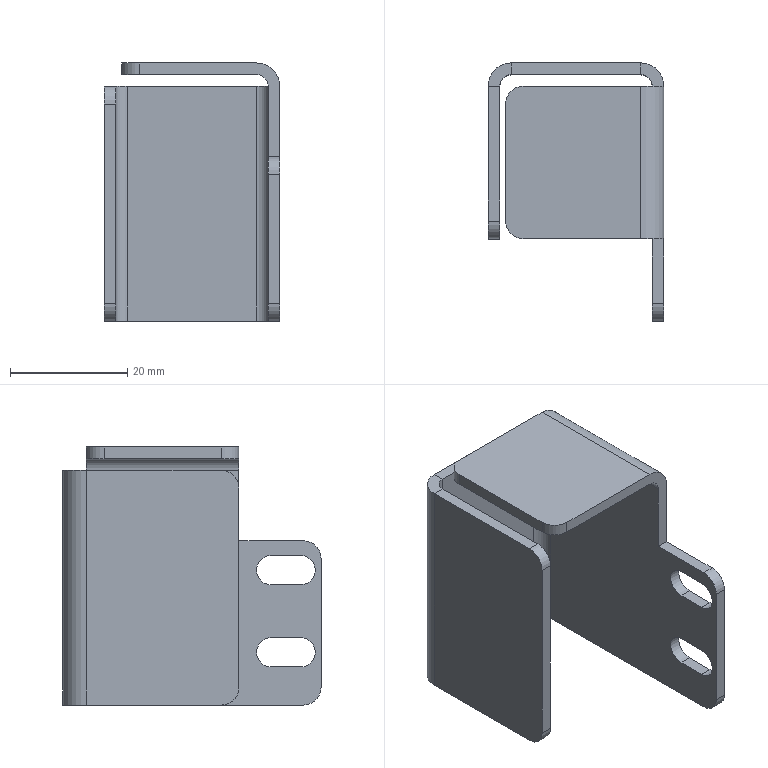Part | NX | features BREP 1 | 1 solid | 44 faces | box 30 x 44 x 44 mm | volume 8697 mm3 | plane 28 | cylinder 16 | commonest cylinder face diameters 6 x6 5 x4 4 x3 8 x3
STEP:
#1=CARTESIAN_POINT('',(-2.,42.,40.));
#2=VERTEX_POINT('',#1);
#3=CARTESIAN_POINT('',(-2.,44.,40.));
#4=VERTEX_POINT('',#3);
#5=CARTESIAN_POINT('',(-2.,42.,40.));
#6=DIRECTION('',(0.,1.,0.));
#7=VECTOR('',#6,1000.);
#8=LINE('',#5,#7);
#9=EDGE_CURVE('',#2,#4,#8,.T.);
#10=ORIENTED_EDGE('',*,*,#9,.F.);
#11=CARTESIAN_POINT('',(0.,40.,40.));
#12=VERTEX_POINT('',#11);
#13=CARTESIAN_POINT('',(-2.,40.,40.));
#14=DIRECTION('',(0.,0.,1.));
#15=DIRECTION('',(-1.,0.,0.));
#16=AXIS2_PLACEMENT_3D('',#13,#14,#15);
#17=CIRCLE('',#16,2.);
#18=EDGE_CURVE('',#12,#2,#17,.T.);
#19=ORIENTED_EDGE('',*,*,#18,.F.);
#20=CARTESIAN_POINT('',(2.,40.,40.));
#21=VERTEX_POINT('',#20);
#22=CARTESIAN_POINT('',(2.,40.,40.));
#23=DIRECTION('',(-1.,0.,0.));
#24=VECTOR('',#23,1000.);
#25=LINE('',#22,#24);
#26=EDGE_CURVE('',#21,#12,#25,.T.);
#27=ORIENTED_EDGE('',*,*,#26,.F.);
#28=CARTESIAN_POINT('',(-2.,40.,40.));
#29=DIRECTION('',(0.,0.,1.));
#30=DIRECTION('',(1.,0.,0.));
#31=AXIS2_PLACEMENT_3D('',#28,#29,#30);
#32=CIRCLE('',#31,4.);
#33=EDGE_CURVE('',#21,#4,#32,.T.);
#34=ORIENTED_EDGE('',*,*,#33,.T.);
#35=EDGE_LOOP('',(#10,#19,#27,#34));
#36=FACE_BOUND('',#35,.T.);
#37=CARTESIAN_POINT('',(-2.,42.,40.));
#38=DIRECTION('',(0.,0.,1.));
#39=DIRECTION('',(-1.,0.,0.));
#40=AXIS2_PLACEMENT_3D('',#37,#38,#39);
#41=PLANE('',#40);
#42=ADVANCED_FACE('',(#36),#41,.T.);
#43=CARTESIAN_POINT('',(-24.,42.,40.));
#44=VERTEX_POINT('',#43);
#45=CARTESIAN_POINT('',(0.,42.,40.));
#46=DIRECTION('',(-1.,0.,0.));
#47=VECTOR('',#46,1000.);
#48=LINE('',#45,#47);
#49=EDGE_CURVE('',#2,#44,#48,.T.);
#50=ORIENTED_EDGE('',*,*,#49,.F.);
#51=ORIENTED_EDGE('',*,*,#9,.T.);
#52=CARTESIAN_POINT('',(-24.,44.,40.));
#53=VERTEX_POINT('',#52);
#54=CARTESIAN_POINT('',(0.,44.,40.));
#55=DIRECTION('',(-1.,0.,0.));
#56=VECTOR('',#55,1000.);
#57=LINE('',#54,#56);
#58=EDGE_CURVE('',#4,#53,#57,.T.);
#59=ORIENTED_EDGE('',*,*,#58,.T.);
#60=CARTESIAN_POINT('',(-24.,44.,40.));
#61=DIRECTION('',(0.,-1.,0.));
#62=VECTOR('',#61,1000.);
#63=LINE('',#60,#62);
#64=EDGE_CURVE('',#53,#44,#63,.T.);
#65=ORIENTED_EDGE('',*,*,#64,.T.);
#66=EDGE_LOOP('',(#50,#51,#59,#65));
#67=FACE_BOUND('',#66,.T.);
#68=CARTESIAN_POINT('',(2.,40.,40.));
#69=DIRECTION('',(0.,0.,1.));
#70=DIRECTION('',(-1.,0.,0.));
#71=AXIS2_PLACEMENT_3D('',#68,#69,#70);
#72=PLANE('',#71);
#73=ADVANCED_FACE('',(#67),#72,.T.);
#74=CARTESIAN_POINT('',(0.,40.,0.));
#75=VERTEX_POINT('',#74);
#76=CARTESIAN_POINT('',(2.,40.,0.));
#77=VERTEX_POINT('',#76);
#78=CARTESIAN_POINT('',(0.,40.,0.));
#79=DIRECTION('',(1.,0.,0.));
#80=VECTOR('',#79,1000.);
#81=LINE('',#78,#80);
#82=EDGE_CURVE('',#75,#77,#81,.T.);
#83=ORIENTED_EDGE('',*,*,#82,.F.);
#84=CARTESIAN_POINT('',(-2.,42.,0.));
#85=VERTEX_POINT('',#84);
#86=CARTESIAN_POINT('',(-2.,40.,0.));
#87=DIRECTION('',(0.,0.,1.));
#88=DIRECTION('',(-1.,0.,0.));
#89=AXIS2_PLACEMENT_3D('',#86,#87,#88);
#90=CIRCLE('',#89,2.);
#91=EDGE_CURVE('',#75,#85,#90,.T.);
#92=ORIENTED_EDGE('',*,*,#91,.T.);
#93=CARTESIAN_POINT('',(-2.,44.,0.));
#94=VERTEX_POINT('',#93);
#95=CARTESIAN_POINT('',(-2.,44.,0.));
#96=DIRECTION('',(0.,-1.,0.));
#97=VECTOR('',#96,1000.);
#98=LINE('',#95,#97);
#99=EDGE_CURVE('',#94,#85,#98,.T.);
#100=ORIENTED_EDGE('',*,*,#99,.F.);
#101=CARTESIAN_POINT('',(-2.,40.,0.));
#102=DIRECTION('',(0.,0.,1.));
#103=DIRECTION('',(1.,0.,0.));
#104=AXIS2_PLACEMENT_3D('',#101,#102,#103);
#105=CIRCLE('',#104,4.);
#106=EDGE_CURVE('',#77,#94,#105,.T.);
#107=ORIENTED_EDGE('',*,*,#106,.F.);
#108=EDGE_LOOP('',(#83,#92,#100,#107));
#109=FACE_BOUND('',#108,.T.);
#110=CARTESIAN_POINT('',(0.,40.,0.));
#111=DIRECTION('',(0.,0.,-1.));
#112=DIRECTION('',(1.,0.,0.));
#113=AXIS2_PLACEMENT_3D('',#110,#111,#112);
#114=PLANE('',#113);
#115=ADVANCED_FACE('',(#109),#114,.T.);
#116=CARTESIAN_POINT('',(2.,3.,0.));
#117=VERTEX_POINT('',#116);
#118=CARTESIAN_POINT('',(2.,0.,0.));
#119=DIRECTION('',(0.,1.,0.));
#120=VECTOR('',#119,1000.);
#121=LINE('',#118,#120);
#122=EDGE_CURVE('',#117,#77,#121,.T.);
#123=ORIENTED_EDGE('',*,*,#122,.F.);
#124=CARTESIAN_POINT('',(0.,3.,0.));
#125=VERTEX_POINT('',#124);
#126=CARTESIAN_POINT('',(-2.,3.,0.));
#127=DIRECTION('',(-1.,0.,0.));
#128=VECTOR('',#127,1000.);
#129=LINE('',#126,#128);
#130=EDGE_CURVE('',#117,#125,#129,.T.);
#131=ORIENTED_EDGE('',*,*,#130,.T.);
#132=CARTESIAN_POINT('',(0.,0.,0.));
#133=DIRECTION('',(0.,1.,0.));
#134=VECTOR('',#133,1000.);
#135=LINE('',#132,#134);
#136=EDGE_CURVE('',#125,#75,#135,.T.);
#137=ORIENTED_EDGE('',*,*,#136,.T.);
#138=ORIENTED_EDGE('',*,*,#82,.T.);
#139=EDGE_LOOP('',(#123,#131,#137,#138));
#140=FACE_BOUND('',#139,.T.);
#141=CARTESIAN_POINT('',(-2.,44.,0.));
#142=DIRECTION('',(0.,0.,-1.));
#143=DIRECTION('',(1.,0.,0.));
#144=AXIS2_PLACEMENT_3D('',#141,#142,#143);
#145=PLANE('',#144);
#146=ADVANCED_FACE('',(#140),#145,.T.);
#147=CARTESIAN_POINT('',(-26.,40.,40.));
#148=VERTEX_POINT('',#147);
#149=CARTESIAN_POINT('',(-28.,40.,40.));
#150=VERTEX_POINT('',#149);
#151=CARTESIAN_POINT('',(-26.,40.,40.));
#152=DIRECTION('',(-1.,0.,0.));
#153=VECTOR('',#152,1000.);
#154=LINE('',#151,#153);
#155=EDGE_CURVE('',#148,#150,#154,.T.);
#156=ORIENTED_EDGE('',*,*,#155,.F.);
#157=CARTESIAN_POINT('',(-24.,40.,40.));
#158=DIRECTION('',(0.,0.,1.));
#159=DIRECTION('',(-1.,0.,0.));
#160=AXIS2_PLACEMENT_3D('',#157,#158,#159);
#161=CIRCLE('',#160,2.);
#162=EDGE_CURVE('',#44,#148,#161,.T.);
#163=ORIENTED_EDGE('',*,*,#162,.F.);
#164=ORIENTED_EDGE('',*,*,#64,.F.);
#165=CARTESIAN_POINT('',(-24.,40.,40.));
#166=DIRECTION('',(0.,0.,1.));
#167=DIRECTION('',(1.,0.,0.));
#168=AXIS2_PLACEMENT_3D('',#165,#166,#167);
#169=CIRCLE('',#168,4.);
#170=EDGE_CURVE('',#53,#150,#169,.T.);
#171=ORIENTED_EDGE('',*,*,#170,.T.);
#172=EDGE_LOOP('',(#156,#163,#164,#171));
#173=FACE_BOUND('',#172,.T.);
#174=CARTESIAN_POINT('',(-26.,40.,40.));
#175=DIRECTION('',(0.,0.,1.));
#176=DIRECTION('',(-1.,0.,0.));
#177=AXIS2_PLACEMENT_3D('',#174,#175,#176);
#178=PLANE('',#177);
#179=ADVANCED_FACE('',(#173),#178,.T.);
#180=CARTESIAN_POINT('',(-28.,17.,40.));
#181=VERTEX_POINT('',#180);
#182=CARTESIAN_POINT('',(-28.,42.,40.));
#183=DIRECTION('',(0.,-1.,0.));
#184=VECTOR('',#183,1000.);
#185=LINE('',#182,#184);
#186=EDGE_CURVE('',#150,#181,#185,.T.);
#187=ORIENTED_EDGE('',*,*,#186,.T.);
#188=CARTESIAN_POINT('',(-26.,17.,40.));
#189=VERTEX_POINT('',#188);
#190=CARTESIAN_POINT('',(-24.,17.,40.));
#191=DIRECTION('',(1.,0.,0.));
#192=VECTOR('',#191,1000.);
#193=LINE('',#190,#192);
#194=EDGE_CURVE('',#181,#189,#193,.T.);
#195=ORIENTED_EDGE('',*,*,#194,.T.);
#196=CARTESIAN_POINT('',(-26.,42.,40.));
#197=DIRECTION('',(0.,-1.,0.));
#198=VECTOR('',#197,1000.);
#199=LINE('',#196,#198);
#200=EDGE_CURVE('',#148,#189,#199,.T.);
#201=ORIENTED_EDGE('',*,*,#200,.F.);
#202=ORIENTED_EDGE('',*,*,#155,.T.);
#203=EDGE_LOOP('',(#187,#195,#201,#202));
#204=FACE_BOUND('',#203,.T.);
#205=CARTESIAN_POINT('',(-24.,44.,40.));
#206=DIRECTION('',(0.,0.,1.));
#207=DIRECTION('',(-1.,0.,0.));
#208=AXIS2_PLACEMENT_3D('',#205,#206,#207);
#209=PLANE('',#208);
#210=ADVANCED_FACE('',(#204),#209,.T.);
#211=CARTESIAN_POINT('',(-24.,42.,0.));
#212=VERTEX_POINT('',#211);
#213=CARTESIAN_POINT('',(-24.,44.,0.));
#214=VERTEX_POINT('',#213);
#215=CARTESIAN_POINT('',(-24.,42.,0.));
#216=DIRECTION('',(0.,1.,0.));
#217=VECTOR('',#216,1000.);
#218=LINE('',#215,#217);
#219=EDGE_CURVE('',#212,#214,#218,.T.);
#220=ORIENTED_EDGE('',*,*,#219,.F.);
#221=CARTESIAN_POINT('',(-26.,40.,0.));
#222=VERTEX_POINT('',#221);
#223=CARTESIAN_POINT('',(-24.,40.,0.));
#224=DIRECTION('',(0.,0.,1.));
#225=DIRECTION('',(-1.,0.,0.));
#226=AXIS2_PLACEMENT_3D('',#223,#224,#225);
#227=CIRCLE('',#226,2.);
#228=EDGE_CURVE('',#212,#222,#227,.T.);
#229=ORIENTED_EDGE('',*,*,#228,.T.);
#230=CARTESIAN_POINT('',(-28.,40.,0.));
#231=VERTEX_POINT('',#230);
#232=CARTESIAN_POINT('',(-28.,40.,0.));
#233=DIRECTION('',(1.,0.,0.));
#234=VECTOR('',#233,1000.);
#235=LINE('',#232,#234);
#236=EDGE_CURVE('',#231,#222,#235,.T.);
#237=ORIENTED_EDGE('',*,*,#236,.F.);
#238=CARTESIAN_POINT('',(-24.,40.,0.));
#239=DIRECTION('',(0.,0.,1.));
#240=DIRECTION('',(1.,0.,0.));
#241=AXIS2_PLACEMENT_3D('',#238,#239,#240);
#242=CIRCLE('',#241,4.);
#243=EDGE_CURVE('',#214,#231,#242,.T.);
#244=ORIENTED_EDGE('',*,*,#243,.F.);
#245=EDGE_LOOP('',(#220,#229,#237,#244));
#246=FACE_BOUND('',#245,.T.);
#247=CARTESIAN_POINT('',(-24.,42.,0.));
#248=DIRECTION('',(0.,0.,-1.));
#249=DIRECTION('',(1.,0.,0.));
#250=AXIS2_PLACEMENT_3D('',#247,#248,#249);
#251=PLANE('',#250);
#252=ADVANCED_FACE('',(#246),#251,.T.);
#253=CARTESIAN_POINT('',(0.,42.,0.));
#254=DIRECTION('',(-1.,0.,0.));
#255=VECTOR('',#254,1000.);
#256=LINE('',#253,#255);
#257=EDGE_CURVE('',#85,#212,#256,.T.);
#258=ORIENTED_EDGE('',*,*,#257,.T.);
#259=ORIENTED_EDGE('',*,*,#219,.T.);
#260=CARTESIAN_POINT('',(0.,44.,0.));
#261=DIRECTION('',(-1.,0.,0.));
#262=VECTOR('',#261,1000.);
#263=LINE('',#260,#262);
#264=EDGE_CURVE('',#94,#214,#263,.T.);
#265=ORIENTED_EDGE('',*,*,#264,.F.);
#266=ORIENTED_EDGE('',*,*,#99,.T.);
#267=EDGE_LOOP('',(#258,#259,#265,#266));
#268=FACE_BOUND('',#267,.T.);
#269=CARTESIAN_POINT('',(-28.,40.,0.));
#270=DIRECTION('',(0.,0.,-1.));
#271=DIRECTION('',(1.,0.,0.));
#272=AXIS2_PLACEMENT_3D('',#269,#270,#271);
#273=PLANE('',#272);
#274=ADVANCED_FACE('',(#268),#273,.T.);
#275=CARTESIAN_POINT('',(-28.,14.,37.));
#276=VERTEX_POINT('',#275);
#277=CARTESIAN_POINT('',(-28.,14.,3.));
#278=VERTEX_POINT('',#277);
#279=CARTESIAN_POINT('',(-28.,14.,40.));
#280=DIRECTION('',(0.,0.,-1.));
#281=VECTOR('',#280,1000.);
#282=LINE('',#279,#281);
#283=EDGE_CURVE('',#276,#278,#282,.T.);
#284=ORIENTED_EDGE('',*,*,#283,.F.);
#285=CARTESIAN_POINT('',(-28.,17.,37.));
#286=DIRECTION('',(-1.,0.,0.));
#287=DIRECTION('',(0.,0.,-1.));
#288=AXIS2_PLACEMENT_3D('',#285,#286,#287);
#289=CIRCLE('',#288,3.);
#290=EDGE_CURVE('',#276,#181,#289,.T.);
#291=ORIENTED_EDGE('',*,*,#290,.T.);
#292=ORIENTED_EDGE('',*,*,#186,.F.);
#293=CARTESIAN_POINT('',(-28.,40.,40.));
#294=DIRECTION('',(0.,0.,-1.));
#295=VECTOR('',#294,1000.);
#296=LINE('',#293,#295);
#297=EDGE_CURVE('',#150,#231,#296,.T.);
#298=ORIENTED_EDGE('',*,*,#297,.T.);
#299=CARTESIAN_POINT('',(-28.,17.,0.));
#300=VERTEX_POINT('',#299);
#301=CARTESIAN_POINT('',(-28.,42.,0.));
#302=DIRECTION('',(0.,-1.,0.));
#303=VECTOR('',#302,1000.);
#304=LINE('',#301,#303);
#305=EDGE_CURVE('',#231,#300,#304,.T.);
#306=ORIENTED_EDGE('',*,*,#305,.T.);
#307=CARTESIAN_POINT('',(-28.,17.,3.));
#308=DIRECTION('',(-1.,0.,0.));
#309=DIRECTION('',(0.,0.,-1.));
#310=AXIS2_PLACEMENT_3D('',#307,#308,#309);
#311=CIRCLE('',#310,3.);
#312=EDGE_CURVE('',#300,#278,#311,.T.);
#313=ORIENTED_EDGE('',*,*,#312,.T.);
#314=EDGE_LOOP('',(#284,#291,#292,#298,#306,#313));
#315=FACE_BOUND('',#314,.T.);
#316=CARTESIAN_POINT('',(-28.,42.,40.));
#317=DIRECTION('',(1.,0.,0.));
#318=DIRECTION('',(0.,0.,1.));
#319=AXIS2_PLACEMENT_3D('',#316,#317,#318);
#320=PLANE('',#319);
#321=ADVANCED_FACE('',(#315),#320,.F.);
#322=CARTESIAN_POINT('',(-26.,14.,37.));
#323=VERTEX_POINT('',#322);
#324=CARTESIAN_POINT('',(-26.,14.,3.));
#325=VERTEX_POINT('',#324);
#326=CARTESIAN_POINT('',(-26.,14.,40.));
#327=DIRECTION('',(0.,0.,-1.));
#328=VECTOR('',#327,1000.);
#329=LINE('',#326,#328);
#330=EDGE_CURVE('',#323,#325,#329,.T.);
#331=ORIENTED_EDGE('',*,*,#330,.F.);
#332=CARTESIAN_POINT('',(-26.,14.,37.));
#333=DIRECTION('',(-1.,0.,0.));
#334=VECTOR('',#333,1000.);
#335=LINE('',#332,#334);
#336=EDGE_CURVE('',#323,#276,#335,.T.);
#337=ORIENTED_EDGE('',*,*,#336,.T.);
#338=ORIENTED_EDGE('',*,*,#283,.T.);
#339=CARTESIAN_POINT('',(-26.,14.,3.));
#340=DIRECTION('',(1.,0.,0.));
#341=VECTOR('',#340,1000.);
#342=LINE('',#339,#341);
#343=EDGE_CURVE('',#278,#325,#342,.T.);
#344=ORIENTED_EDGE('',*,*,#343,.T.);
#345=EDGE_LOOP('',(#331,#337,#338,#344));
#346=FACE_BOUND('',#345,.T.);
#347=CARTESIAN_POINT('',(-26.,14.,40.));
#348=DIRECTION('',(0.,-1.,0.));
#349=DIRECTION('',(0.,0.,1.));
#350=AXIS2_PLACEMENT_3D('',#347,#348,#349);
#351=PLANE('',#350);
#352=ADVANCED_FACE('',(#346),#351,.T.);
#353=ORIENTED_EDGE('',*,*,#200,.T.);
#354=CARTESIAN_POINT('',(-26.,17.,37.));
#355=DIRECTION('',(1.,0.,0.));
#356=DIRECTION('',(0.,0.,-1.));
#357=AXIS2_PLACEMENT_3D('',#354,#355,#356);
#358=CIRCLE('',#357,3.);
#359=EDGE_CURVE('',#189,#323,#358,.T.);
#360=ORIENTED_EDGE('',*,*,#359,.T.);
#361=ORIENTED_EDGE('',*,*,#330,.T.);
#362=CARTESIAN_POINT('',(-26.,17.,0.));
#363=VERTEX_POINT('',#362);
#364=CARTESIAN_POINT('',(-26.,17.,3.));
#365=DIRECTION('',(1.,0.,0.));
#366=DIRECTION('',(0.,0.,-1.));
#367=AXIS2_PLACEMENT_3D('',#364,#365,#366);
#368=CIRCLE('',#367,3.);
#369=EDGE_CURVE('',#325,#363,#368,.T.);
#370=ORIENTED_EDGE('',*,*,#369,.T.);
#371=CARTESIAN_POINT('',(-26.,42.,0.));
#372=DIRECTION('',(0.,-1.,0.));
#373=VECTOR('',#372,1000.);
#374=LINE('',#371,#373);
#375=EDGE_CURVE('',#222,#363,#374,.T.);
#376=ORIENTED_EDGE('',*,*,#375,.F.);
#377=CARTESIAN_POINT('',(-26.,40.,40.));
#378=DIRECTION('',(0.,0.,-1.));
#379=VECTOR('',#378,1000.);
#380=LINE('',#377,#379);
#381=EDGE_CURVE('',#148,#222,#380,.T.);
#382=ORIENTED_EDGE('',*,*,#381,.F.);
#383=EDGE_LOOP('',(#353,#360,#361,#370,#376,#382));
#384=FACE_BOUND('',#383,.T.);
#385=CARTESIAN_POINT('',(-26.,42.,40.));
#386=DIRECTION('',(1.,0.,0.));
#387=DIRECTION('',(0.,0.,1.));
#388=AXIS2_PLACEMENT_3D('',#385,#386,#387);
#389=PLANE('',#388);
#390=ADVANCED_FACE('',(#384),#389,.T.);
#391=ORIENTED_EDGE('',*,*,#228,.F.);
#392=CARTESIAN_POINT('',(-24.,42.,40.));
#393=DIRECTION('',(0.,0.,-1.));
#394=VECTOR('',#393,1000.);
#395=LINE('',#392,#394);
#396=EDGE_CURVE('',#44,#212,#395,.T.);
#397=ORIENTED_EDGE('',*,*,#396,.F.);
#398=ORIENTED_EDGE('',*,*,#162,.T.);
#399=ORIENTED_EDGE('',*,*,#381,.T.);
#400=EDGE_LOOP('',(#391,#397,#398,#399));
#401=FACE_BOUND('',#400,.T.);
#402=CARTESIAN_POINT('',(-24.,40.,40.));
#403=DIRECTION('',(0.,0.,-1.));
#404=DIRECTION('',(1.,0.,0.));
#405=AXIS2_PLACEMENT_3D('',#402,#403,#404);
#406=CYLINDRICAL_SURFACE('',#405,2.);
#407=ADVANCED_FACE('',(#401),#406,.F.);
#408=ORIENTED_EDGE('',*,*,#257,.F.);
#409=CARTESIAN_POINT('',(-2.,42.,40.));
#410=DIRECTION('',(0.,0.,-1.));
#411=VECTOR('',#410,1000.);
#412=LINE('',#409,#411);
#413=EDGE_CURVE('',#2,#85,#412,.T.);
#414=ORIENTED_EDGE('',*,*,#413,.F.);
#415=ORIENTED_EDGE('',*,*,#49,.T.);
#416=ORIENTED_EDGE('',*,*,#396,.T.);
#417=EDGE_LOOP('',(#408,#414,#415,#416));
#418=FACE_BOUND('',#417,.T.);
#419=CARTESIAN_POINT('',(0.,42.,40.));
#420=DIRECTION('',(0.,-1.,0.));
#421=DIRECTION('',(-1.,0.,0.));
#422=AXIS2_PLACEMENT_3D('',#419,#420,#421);
#423=PLANE('',#422);
#424=ADVANCED_FACE('',(#418),#423,.T.);
#425=ORIENTED_EDGE('',*,*,#91,.F.);
#426=CARTESIAN_POINT('',(0.,40.,40.));
#427=DIRECTION('',(0.,0.,-1.));
#428=VECTOR('',#427,1000.);
#429=LINE('',#426,#428);
#430=EDGE_CURVE('',#12,#75,#429,.T.);
#431=ORIENTED_EDGE('',*,*,#430,.F.);
#432=ORIENTED_EDGE('',*,*,#18,.T.);
#433=ORIENTED_EDGE('',*,*,#413,.T.);
#434=EDGE_LOOP('',(#425,#431,#432,#433));
#435=FACE_BOUND('',#434,.T.);
#436=CARTESIAN_POINT('',(-2.,40.,40.));
#437=DIRECTION('',(0.,0.,-1.));
#438=DIRECTION('',(1.,0.,0.));
#439=AXIS2_PLACEMENT_3D('',#436,#437,#438);
#440=CYLINDRICAL_SURFACE('',#439,2.);
#441=ADVANCED_FACE('',(#435),#440,.F.);
#442=CARTESIAN_POINT('',(0.,8.5,25.5));
#443=VERTEX_POINT('',#442);
#444=CARTESIAN_POINT('',(0.,8.5,20.5));
#445=VERTEX_POINT('',#444);
#446=CARTESIAN_POINT('',(0.,8.5,23.));
#447=DIRECTION('',(-1.,0.,0.));
#448=DIRECTION('',(0.,0.,1.));
#449=AXIS2_PLACEMENT_3D('',#446,#447,#448);
#450=CIRCLE('',#449,2.5);
#451=EDGE_CURVE('',#443,#445,#450,.T.);
#452=ORIENTED_EDGE('',*,*,#451,.F.);
#453=CARTESIAN_POINT('',(0.,3.5,25.5));
#454=VERTEX_POINT('',#453);
#455=CARTESIAN_POINT('',(0.,0.,25.5));
#456=DIRECTION('',(0.,1.,0.));
#457=VECTOR('',#456,1000.);
#458=LINE('',#455,#457);
#459=EDGE_CURVE('',#454,#443,#458,.T.);
#460=ORIENTED_EDGE('',*,*,#459,.F.);
#461=CARTESIAN_POINT('',(0.,3.5,20.5));
#462=VERTEX_POINT('',#461);
#463=CARTESIAN_POINT('',(0.,3.5,23.));
#464=DIRECTION('',(-1.,0.,0.));
#465=DIRECTION('',(0.,0.,1.));
#466=AXIS2_PLACEMENT_3D('',#463,#464,#465);
#467=CIRCLE('',#466,2.5);
#468=EDGE_CURVE('',#462,#454,#467,.T.);
#469=ORIENTED_EDGE('',*,*,#468,.F.);
#470=CARTESIAN_POINT('',(0.,0.,20.5));
#471=DIRECTION('',(0.,-1.,0.));
#472=VECTOR('',#471,1000.);
#473=LINE('',#470,#472);
#474=EDGE_CURVE('',#445,#462,#473,.T.);
#475=ORIENTED_EDGE('',*,*,#474,.F.);
#476=EDGE_LOOP('',(#452,#460,#469,#475));
#477=FACE_BOUND('',#476,.T.);
#478=CARTESIAN_POINT('',(0.,8.5,11.5));
#479=VERTEX_POINT('',#478);
#480=CARTESIAN_POINT('',(0.,8.5,6.5));
#481=VERTEX_POINT('',#480);
#482=CARTESIAN_POINT('',(0.,8.5,9.));
#483=DIRECTION('',(-1.,0.,0.));
#484=DIRECTION('',(0.,0.,1.));
#485=AXIS2_PLACEMENT_3D('',#482,#483,#484);
#486=CIRCLE('',#485,2.5);
#487=EDGE_CURVE('',#479,#481,#486,.T.);
#488=ORIENTED_EDGE('',*,*,#487,.F.);
#489=CARTESIAN_POINT('',(0.,3.5,11.5));
#490=VERTEX_POINT('',#489);
#491=CARTESIAN_POINT('',(0.,0.,11.5));
#492=DIRECTION('',(0.,1.,0.));
#493=VECTOR('',#492,1000.);
#494=LINE('',#491,#493);
#495=EDGE_CURVE('',#490,#479,#494,.T.);
#496=ORIENTED_EDGE('',*,*,#495,.F.);
#497=CARTESIAN_POINT('',(0.,3.5,6.5));
#498=VERTEX_POINT('',#497);
#499=CARTESIAN_POINT('',(0.,3.5,9.));
#500=DIRECTION('',(-1.,0.,0.));
#501=DIRECTION('',(0.,0.,1.));
#502=AXIS2_PLACEMENT_3D('',#499,#500,#501);
#503=CIRCLE('',#502,2.5);
#504=EDGE_CURVE('',#498,#490,#503,.T.);
#505=ORIENTED_EDGE('',*,*,#504,.F.);
#506=CARTESIAN_POINT('',(0.,0.,6.5));
#507=DIRECTION('',(0.,-1.,0.));
#508=VECTOR('',#507,1000.);
#509=LINE('',#506,#508);
#510=EDGE_CURVE('',#481,#498,#509,.T.);
#511=ORIENTED_EDGE('',*,*,#510,.F.);
#512=EDGE_LOOP('',(#488,#496,#505,#511));
#513=FACE_BOUND('',#512,.T.);
#514=ORIENTED_EDGE('',*,*,#136,.F.);
#515=CARTESIAN_POINT('',(0.,0.,3.));
#516=VERTEX_POINT('',#515);
#517=CARTESIAN_POINT('',(0.,3.,3.));
#518=DIRECTION('',(-1.,0.,0.));
#519=DIRECTION('',(0.,0.,1.));
#520=AXIS2_PLACEMENT_3D('',#517,#518,#519);
#521=CIRCLE('',#520,3.);
#522=EDGE_CURVE('',#125,#516,#521,.T.);
#523=ORIENTED_EDGE('',*,*,#522,.T.);
#524=CARTESIAN_POINT('',(0.,0.,25.));
#525=VERTEX_POINT('',#524);
#526=CARTESIAN_POINT('',(0.,0.,40.));
#527=DIRECTION('',(0.,0.,-1.));
#528=VECTOR('',#527,1000.);
#529=LINE('',#526,#528);
#530=EDGE_CURVE('',#525,#516,#529,.T.);
#531=ORIENTED_EDGE('',*,*,#530,.F.);
#532=CARTESIAN_POINT('',(0.,3.,28.));
#533=VERTEX_POINT('',#532);
#534=CARTESIAN_POINT('',(0.,3.,25.));
#535=DIRECTION('',(-1.,0.,0.));
#536=DIRECTION('',(0.,0.,1.));
#537=AXIS2_PLACEMENT_3D('',#534,#535,#536);
#538=CIRCLE('',#537,3.);
#539=EDGE_CURVE('',#525,#533,#538,.T.);
#540=ORIENTED_EDGE('',*,*,#539,.T.);
#541=CARTESIAN_POINT('',(0.,14.,28.));
#542=VERTEX_POINT('',#541);
#543=CARTESIAN_POINT('',(0.,0.,28.));
#544=DIRECTION('',(0.,-1.,0.));
#545=VECTOR('',#544,1000.);
#546=LINE('',#543,#545);
#547=EDGE_CURVE('',#542,#533,#546,.T.);
#548=ORIENTED_EDGE('',*,*,#547,.F.);
#549=CARTESIAN_POINT('',(0.,14.,40.));
#550=VERTEX_POINT('',#549);
#551=CARTESIAN_POINT('',(0.,14.,40.));
#552=DIRECTION('',(0.,0.,-1.));
#553=VECTOR('',#552,1000.);
#554=LINE('',#551,#553);
#555=EDGE_CURVE('',#550,#542,#554,.T.);
#556=ORIENTED_EDGE('',*,*,#555,.F.);
#557=CARTESIAN_POINT('',(0.,0.,40.));
#558=DIRECTION('',(0.,1.,0.));
#559=VECTOR('',#558,1000.);
#560=LINE('',#557,#559);
#561=EDGE_CURVE('',#550,#12,#560,.T.);
#562=ORIENTED_EDGE('',*,*,#561,.T.);
#563=ORIENTED_EDGE('',*,*,#430,.T.);
#564=EDGE_LOOP('',(#514,#523,#531,#540,#548,#556,#562,#563));
#565=FACE_BOUND('',#564,.T.);
#566=CARTESIAN_POINT('',(0.,0.,40.));
#567=DIRECTION('',(-1.,0.,0.));
#568=DIRECTION('',(0.,0.,-1.));
#569=AXIS2_PLACEMENT_3D('',#566,#567,#568);
#570=PLANE('',#569);
#571=ADVANCED_FACE('',(#477,#513,#565),#570,.T.);
#572=ORIENTED_EDGE('',*,*,#530,.T.);
#573=CARTESIAN_POINT('',(2.,0.,3.));
#574=VERTEX_POINT('',#573);
#575=CARTESIAN_POINT('',(2.,0.,3.));
#576=DIRECTION('',(1.,0.,0.));
#577=VECTOR('',#576,1000.);
#578=LINE('',#575,#577);
#579=EDGE_CURVE('',#516,#574,#578,.T.);
#580=ORIENTED_EDGE('',*,*,#579,.T.);
#581=CARTESIAN_POINT('',(2.,0.,25.));
#582=VERTEX_POINT('',#581);
#583=CARTESIAN_POINT('',(2.,0.,40.));
#584=DIRECTION('',(0.,0.,-1.));
#585=VECTOR('',#584,1000.);
#586=LINE('',#583,#585);
#587=EDGE_CURVE('',#582,#574,#586,.T.);
#588=ORIENTED_EDGE('',*,*,#587,.F.);
#589=CARTESIAN_POINT('',(0.,0.,25.));
#590=DIRECTION('',(-1.,0.,0.));
#591=VECTOR('',#590,1000.);
#592=LINE('',#589,#591);
#593=EDGE_CURVE('',#582,#525,#592,.T.);
#594=ORIENTED_EDGE('',*,*,#593,.T.);
#595=EDGE_LOOP('',(#572,#580,#588,#594));
#596=FACE_BOUND('',#595,.T.);
#597=CARTESIAN_POINT('',(2.,0.,40.));
#598=DIRECTION('',(0.,-1.,0.));
#599=DIRECTION('',(0.,0.,1.));
#600=AXIS2_PLACEMENT_3D('',#597,#598,#599);
#601=PLANE('',#600);
#602=ADVANCED_FACE('',(#596),#601,.T.);
#603=CARTESIAN_POINT('',(2.,8.5,25.5));
#604=VERTEX_POINT('',#603);
#605=CARTESIAN_POINT('',(2.,3.5,25.5));
#606=VERTEX_POINT('',#605);
#607=CARTESIAN_POINT('',(2.,8.5,25.5));
#608=DIRECTION('',(0.,-1.,0.));
#609=VECTOR('',#608,1000.);
#610=LINE('',#607,#609);
#611=EDGE_CURVE('',#604,#606,#610,.T.);
#612=ORIENTED_EDGE('',*,*,#611,.F.);
#613=CARTESIAN_POINT('',(2.,8.5,20.5));
#614=VERTEX_POINT('',#613);
#615=CARTESIAN_POINT('',(2.,8.5,23.));
#616=DIRECTION('',(1.,0.,0.));
#617=DIRECTION('',(0.,0.,-1.));
#618=AXIS2_PLACEMENT_3D('',#615,#616,#617);
#619=CIRCLE('',#618,2.5);
#620=EDGE_CURVE('',#614,#604,#619,.T.);
#621=ORIENTED_EDGE('',*,*,#620,.F.);
#622=CARTESIAN_POINT('',(2.,3.5,20.5));
#623=VERTEX_POINT('',#622);
#624=CARTESIAN_POINT('',(2.,8.5,20.5));
#625=DIRECTION('',(0.,1.,0.));
#626=VECTOR('',#625,1000.);
#627=LINE('',#624,#626);
#628=EDGE_CURVE('',#623,#614,#627,.T.);
#629=ORIENTED_EDGE('',*,*,#628,.F.);
#630=CARTESIAN_POINT('',(2.,3.5,23.));
#631=DIRECTION('',(1.,0.,0.));
#632=DIRECTION('',(0.,0.,-1.));
#633=AXIS2_PLACEMENT_3D('',#630,#631,#632);
#634=CIRCLE('',#633,2.5);
#635=EDGE_CURVE('',#606,#623,#634,.T.);
#636=ORIENTED_EDGE('',*,*,#635,.F.);
#637=EDGE_LOOP('',(#612,#621,#629,#636));
#638=FACE_BOUND('',#637,.T.);
#639=CARTESIAN_POINT('',(2.,8.5,11.5));
#640=VERTEX_POINT('',#639);
#641=CARTESIAN_POINT('',(2.,3.5,11.5));
#642=VERTEX_POINT('',#641);
#643=CARTESIAN_POINT('',(2.,8.5,11.5));
#644=DIRECTION('',(0.,-1.,0.));
#645=VECTOR('',#644,1000.);
#646=LINE('',#643,#645);
#647=EDGE_CURVE('',#640,#642,#646,.T.);
#648=ORIENTED_EDGE('',*,*,#647,.F.);
#649=CARTESIAN_POINT('',(2.,8.5,6.5));
#650=VERTEX_POINT('',#649);
#651=CARTESIAN_POINT('',(2.,8.5,9.));
#652=DIRECTION('',(1.,0.,0.));
#653=DIRECTION('',(0.,0.,-1.));
#654=AXIS2_PLACEMENT_3D('',#651,#652,#653);
#655=CIRCLE('',#654,2.5);
#656=EDGE_CURVE('',#650,#640,#655,.T.);
#657=ORIENTED_EDGE('',*,*,#656,.F.);
#658=CARTESIAN_POINT('',(2.,3.5,6.5));
#659=VERTEX_POINT('',#658);
#660=CARTESIAN_POINT('',(2.,8.5,6.5));
#661=DIRECTION('',(0.,1.,0.));
#662=VECTOR('',#661,1000.);
#663=LINE('',#660,#662);
#664=EDGE_CURVE('',#659,#650,#663,.T.);
#665=ORIENTED_EDGE('',*,*,#664,.F.);
#666=CARTESIAN_POINT('',(2.,3.5,9.));
#667=DIRECTION('',(1.,0.,0.));
#668=DIRECTION('',(0.,0.,-1.));
#669=AXIS2_PLACEMENT_3D('',#666,#667,#668);
#670=CIRCLE('',#669,2.5);
#671=EDGE_CURVE('',#642,#659,#670,.T.);
#672=ORIENTED_EDGE('',*,*,#671,.F.);
#673=EDGE_LOOP('',(#648,#657,#665,#672));
#674=FACE_BOUND('',#673,.T.);
#675=ORIENTED_EDGE('',*,*,#587,.T.);
#676=CARTESIAN_POINT('',(2.,3.,3.));
#677=DIRECTION('',(1.,0.,0.));
#678=DIRECTION('',(0.,0.,1.));
#679=AXIS2_PLACEMENT_3D('',#676,#677,#678);
#680=CIRCLE('',#679,3.);
#681=EDGE_CURVE('',#574,#117,#680,.T.);
#682=ORIENTED_EDGE('',*,*,#681,.T.);
#683=ORIENTED_EDGE('',*,*,#122,.T.);
#684=CARTESIAN_POINT('',(2.,40.,40.));
#685=DIRECTION('',(0.,0.,-1.));
#686=VECTOR('',#685,1000.);
#687=LINE('',#684,#686);
#688=EDGE_CURVE('',#21,#77,#687,.T.);
#689=ORIENTED_EDGE('',*,*,#688,.F.);
#690=CARTESIAN_POINT('',(2.,14.,40.));
#691=VERTEX_POINT('',#690);
#692=CARTESIAN_POINT('',(2.,0.,40.));
#693=DIRECTION('',(0.,1.,0.));
#694=VECTOR('',#693,1000.);
#695=LINE('',#692,#694);
#696=EDGE_CURVE('',#691,#21,#695,.T.);
#697=ORIENTED_EDGE('',*,*,#696,.F.);
#698=CARTESIAN_POINT('',(2.,14.,28.));
#699=VERTEX_POINT('',#698);
#700=CARTESIAN_POINT('',(2.,14.,28.));
#701=DIRECTION('',(0.,0.,1.));
#702=VECTOR('',#701,1000.);
#703=LINE('',#700,#702);
#704=EDGE_CURVE('',#699,#691,#703,.T.);
#705=ORIENTED_EDGE('',*,*,#704,.F.);
#706=CARTESIAN_POINT('',(2.,3.,28.));
#707=VERTEX_POINT('',#706);
#708=CARTESIAN_POINT('',(2.,14.,28.));
#709=DIRECTION('',(0.,1.,0.));
#710=VECTOR('',#709,1000.);
#711=LINE('',#708,#710);
#712=EDGE_CURVE('',#707,#699,#711,.T.);
#713=ORIENTED_EDGE('',*,*,#712,.F.);
#714=CARTESIAN_POINT('',(2.,3.,25.));
#715=DIRECTION('',(1.,0.,0.));
#716=DIRECTION('',(0.,0.,1.));
#717=AXIS2_PLACEMENT_3D('',#714,#715,#716);
#718=CIRCLE('',#717,3.);
#719=EDGE_CURVE('',#707,#582,#718,.T.);
#720=ORIENTED_EDGE('',*,*,#719,.T.);
#721=EDGE_LOOP('',(#675,#682,#683,#689,#697,#705,#713,#720));
#722=FACE_BOUND('',#721,.T.);
#723=CARTESIAN_POINT('',(2.,0.,40.));
#724=DIRECTION('',(-1.,0.,0.));
#725=DIRECTION('',(0.,0.,-1.));
#726=AXIS2_PLACEMENT_3D('',#723,#724,#725);
#727=PLANE('',#726);
#728=ADVANCED_FACE('',(#638,#674,#722),#727,.F.);
#729=ORIENTED_EDGE('',*,*,#106,.T.);
#730=CARTESIAN_POINT('',(-2.,44.,40.));
#731=DIRECTION('',(0.,0.,-1.));
#732=VECTOR('',#731,1000.);
#733=LINE('',#730,#732);
#734=EDGE_CURVE('',#4,#94,#733,.T.);
#735=ORIENTED_EDGE('',*,*,#734,.F.);
#736=ORIENTED_EDGE('',*,*,#33,.F.);
#737=ORIENTED_EDGE('',*,*,#688,.T.);
#738=EDGE_LOOP('',(#729,#735,#736,#737));
#739=FACE_BOUND('',#738,.T.);
#740=CARTESIAN_POINT('',(-2.,40.,40.));
#741=DIRECTION('',(0.,0.,-1.));
#742=DIRECTION('',(1.,0.,0.));
#743=AXIS2_PLACEMENT_3D('',#740,#741,#742);
#744=CYLINDRICAL_SURFACE('',#743,4.);
#745=ADVANCED_FACE('',(#739),#744,.T.);
#746=ORIENTED_EDGE('',*,*,#264,.T.);
#747=CARTESIAN_POINT('',(-24.,44.,40.));
#748=DIRECTION('',(0.,0.,-1.));
#749=VECTOR('',#748,1000.);
#750=LINE('',#747,#749);
#751=EDGE_CURVE('',#53,#214,#750,.T.);
#752=ORIENTED_EDGE('',*,*,#751,.F.);
#753=ORIENTED_EDGE('',*,*,#58,.F.);
#754=ORIENTED_EDGE('',*,*,#734,.T.);
#755=EDGE_LOOP('',(#746,#752,#753,#754));
#756=FACE_BOUND('',#755,.T.);
#757=CARTESIAN_POINT('',(0.,44.,40.));
#758=DIRECTION('',(0.,-1.,0.));
#759=DIRECTION('',(-1.,0.,0.));
#760=AXIS2_PLACEMENT_3D('',#757,#758,#759);
#761=PLANE('',#760);
#762=ADVANCED_FACE('',(#756),#761,.F.);
#763=ORIENTED_EDGE('',*,*,#243,.T.);
#764=ORIENTED_EDGE('',*,*,#297,.F.);
#765=ORIENTED_EDGE('',*,*,#170,.F.);
#766=ORIENTED_EDGE('',*,*,#751,.T.);
#767=EDGE_LOOP('',(#763,#764,#765,#766));
#768=FACE_BOUND('',#767,.T.);
#769=CARTESIAN_POINT('',(-24.,40.,40.));
#770=DIRECTION('',(0.,0.,-1.));
#771=DIRECTION('',(1.,0.,0.));
#772=AXIS2_PLACEMENT_3D('',#769,#770,#771);
#773=CYLINDRICAL_SURFACE('',#772,4.);
#774=ADVANCED_FACE('',(#768),#773,.T.);
#775=ORIENTED_EDGE('',*,*,#375,.T.);
#776=CARTESIAN_POINT('',(-24.,17.,0.));
#777=DIRECTION('',(-1.,0.,0.));
#778=VECTOR('',#777,1000.);
#779=LINE('',#776,#778);
#780=EDGE_CURVE('',#363,#300,#779,.T.);
#781=ORIENTED_EDGE('',*,*,#780,.T.);
#782=ORIENTED_EDGE('',*,*,#305,.F.);
#783=ORIENTED_EDGE('',*,*,#236,.T.);
#784=EDGE_LOOP('',(#775,#781,#782,#783));
#785=FACE_BOUND('',#784,.T.);
#786=CARTESIAN_POINT('',(-24.,40.,0.));
#787=DIRECTION('',(0.,0.,-1.));
#788=DIRECTION('',(1.,0.,0.));
#789=AXIS2_PLACEMENT_3D('',#786,#787,#788);
#790=PLANE('',#789);
#791=ADVANCED_FACE('',(#785),#790,.T.);
#792=CARTESIAN_POINT('',(-2.,40.,42.));
#793=VERTEX_POINT('',#792);
#794=CARTESIAN_POINT('',(-2.,40.,40.));
#795=DIRECTION('',(0.,1.,0.));
#796=DIRECTION('',(0.,0.,1.));
#797=AXIS2_PLACEMENT_3D('',#794,#795,#796);
#798=CIRCLE('',#797,2.);
#799=EDGE_CURVE('',#793,#12,#798,.T.);
#800=ORIENTED_EDGE('',*,*,#799,.F.);
#801=CARTESIAN_POINT('',(-2.,40.,44.));
#802=VERTEX_POINT('',#801);
#803=CARTESIAN_POINT('',(-2.,40.,42.));
#804=DIRECTION('',(0.,0.,1.));
#805=VECTOR('',#804,1000.);
#806=LINE('',#803,#805);
#807=EDGE_CURVE('',#793,#802,#806,.T.);
#808=ORIENTED_EDGE('',*,*,#807,.T.);
#809=CARTESIAN_POINT('',(-2.,40.,40.));
#810=DIRECTION('',(0.,1.,0.));
#811=DIRECTION('',(0.,0.,1.));
#812=AXIS2_PLACEMENT_3D('',#809,#810,#811);
#813=CIRCLE('',#812,4.);
#814=EDGE_CURVE('',#802,#21,#813,.T.);
#815=ORIENTED_EDGE('',*,*,#814,.T.);
#816=ORIENTED_EDGE('',*,*,#26,.T.);
#817=EDGE_LOOP('',(#800,#808,#815,#816));
#818=FACE_BOUND('',#817,.T.);
#819=CARTESIAN_POINT('',(-2.,40.,40.));
#820=DIRECTION('',(0.,-1.,0.));
#821=DIRECTION('',(0.,0.,1.));
#822=AXIS2_PLACEMENT_3D('',#819,#820,#821);
#823=PLANE('',#822);
#824=ADVANCED_FACE('',(#818),#823,.F.);
#825=CARTESIAN_POINT('',(-2.,14.,44.));
#826=VERTEX_POINT('',#825);
#827=CARTESIAN_POINT('',(-2.,14.,40.));
#828=DIRECTION('',(0.,-1.,0.));
#829=DIRECTION('',(-1.,0.,0.));
#830=AXIS2_PLACEMENT_3D('',#827,#828,#829);
#831=CIRCLE('',#830,4.);
#832=EDGE_CURVE('',#691,#826,#831,.T.);
#833=ORIENTED_EDGE('',*,*,#832,.F.);
#834=ORIENTED_EDGE('',*,*,#696,.T.);
#835=ORIENTED_EDGE('',*,*,#814,.F.);
#836=CARTESIAN_POINT('',(-2.,0.,44.));
#837=DIRECTION('',(0.,-1.,0.));
#838=VECTOR('',#837,1000.);
#839=LINE('',#836,#838);
#840=EDGE_CURVE('',#802,#826,#839,.T.);
#841=ORIENTED_EDGE('',*,*,#840,.T.);
#842=EDGE_LOOP('',(#833,#834,#835,#841));
#843=FACE_BOUND('',#842,.T.);
#844=CARTESIAN_POINT('',(-2.,40.,40.));
#845=DIRECTION('',(0.,1.,0.));
#846=DIRECTION('',(0.,0.,-1.));
#847=AXIS2_PLACEMENT_3D('',#844,#845,#846);
#848=CYLINDRICAL_SURFACE('',#847,4.);
#849=ADVANCED_FACE('',(#843),#848,.T.);
#850=ORIENTED_EDGE('',*,*,#561,.F.);
#851=CARTESIAN_POINT('',(-2.,14.,42.));
#852=VERTEX_POINT('',#851);
#853=CARTESIAN_POINT('',(-2.,14.,40.));
#854=DIRECTION('',(0.,-1.,0.));
#855=DIRECTION('',(-1.,0.,0.));
#856=AXIS2_PLACEMENT_3D('',#853,#854,#855);
#857=CIRCLE('',#856,2.);
#858=EDGE_CURVE('',#550,#852,#857,.T.);
#859=ORIENTED_EDGE('',*,*,#858,.T.);
#860=CARTESIAN_POINT('',(-2.,0.,42.));
#861=DIRECTION('',(0.,1.,0.));
#862=VECTOR('',#861,1000.);
#863=LINE('',#860,#862);
#864=EDGE_CURVE('',#852,#793,#863,.T.);
#865=ORIENTED_EDGE('',*,*,#864,.T.);
#866=ORIENTED_EDGE('',*,*,#799,.T.);
#867=EDGE_LOOP('',(#850,#859,#865,#866));
#868=FACE_BOUND('',#867,.T.);
#869=CARTESIAN_POINT('',(-2.,40.,40.));
#870=DIRECTION('',(0.,1.,0.));
#871=DIRECTION('',(0.,0.,-1.));
#872=AXIS2_PLACEMENT_3D('',#869,#870,#871);
#873=CYLINDRICAL_SURFACE('',#872,2.);
#874=ADVANCED_FACE('',(#868),#873,.F.);
#875=CARTESIAN_POINT('',(-22.,40.,42.));
#876=VERTEX_POINT('',#875);
#877=CARTESIAN_POINT('',(-25.,40.,42.));
#878=DIRECTION('',(-1.,0.,0.));
#879=VECTOR('',#878,1000.);
#880=LINE('',#877,#879);
#881=EDGE_CURVE('',#793,#876,#880,.T.);
#882=ORIENTED_EDGE('',*,*,#881,.T.);
#883=CARTESIAN_POINT('',(-22.,40.,44.));
#884=VERTEX_POINT('',#883);
#885=CARTESIAN_POINT('',(-22.,40.,44.));
#886=DIRECTION('',(0.,0.,1.));
#887=VECTOR('',#886,1000.);
#888=LINE('',#885,#887);
#889=EDGE_CURVE('',#876,#884,#888,.T.);
#890=ORIENTED_EDGE('',*,*,#889,.T.);
#891=CARTESIAN_POINT('',(0.,40.,44.));
#892=DIRECTION('',(-1.,0.,0.));
#893=VECTOR('',#892,1000.);
#894=LINE('',#891,#893);
#895=EDGE_CURVE('',#802,#884,#894,.T.);
#896=ORIENTED_EDGE('',*,*,#895,.F.);
#897=ORIENTED_EDGE('',*,*,#807,.F.);
#898=EDGE_LOOP('',(#882,#890,#896,#897));
#899=FACE_BOUND('',#898,.T.);
#900=CARTESIAN_POINT('',(-25.,40.,44.));
#901=DIRECTION('',(0.,-1.,0.));
#902=DIRECTION('',(0.,0.,1.));
#903=AXIS2_PLACEMENT_3D('',#900,#901,#902);
#904=PLANE('',#903);
#905=ADVANCED_FACE('',(#899),#904,.F.);
#906=ORIENTED_EDGE('',*,*,#895,.T.);
#907=CARTESIAN_POINT('',(-25.,37.,44.));
#908=VERTEX_POINT('',#907);
#909=CARTESIAN_POINT('',(-22.,37.,44.));
#910=DIRECTION('',(0.,0.,1.));
#911=DIRECTION('',(-1.,0.,0.));
#912=AXIS2_PLACEMENT_3D('',#909,#910,#911);
#913=CIRCLE('',#912,3.);
#914=EDGE_CURVE('',#884,#908,#913,.T.);
#915=ORIENTED_EDGE('',*,*,#914,.T.);
#916=CARTESIAN_POINT('',(-25.,17.,44.));
#917=VERTEX_POINT('',#916);
#918=CARTESIAN_POINT('',(-25.,0.,44.));
#919=DIRECTION('',(0.,-1.,0.));
#920=VECTOR('',#919,1000.);
#921=LINE('',#918,#920);
#922=EDGE_CURVE('',#908,#917,#921,.T.);
#923=ORIENTED_EDGE('',*,*,#922,.T.);
#924=CARTESIAN_POINT('',(-22.,14.,44.));
#925=VERTEX_POINT('',#924);
#926=CARTESIAN_POINT('',(-22.,17.,44.));
#927=DIRECTION('',(0.,0.,1.));
#928=DIRECTION('',(-1.,0.,0.));
#929=AXIS2_PLACEMENT_3D('',#926,#927,#928);
#930=CIRCLE('',#929,3.);
#931=EDGE_CURVE('',#917,#925,#930,.T.);
#932=ORIENTED_EDGE('',*,*,#931,.T.);
#933=CARTESIAN_POINT('',(2.,14.,44.));
#934=DIRECTION('',(-1.,0.,0.));
#935=VECTOR('',#934,1000.);
#936=LINE('',#933,#935);
#937=EDGE_CURVE('',#826,#925,#936,.T.);
#938=ORIENTED_EDGE('',*,*,#937,.F.);
#939=ORIENTED_EDGE('',*,*,#840,.F.);
#940=EDGE_LOOP('',(#906,#915,#923,#932,#938,#939));
#941=FACE_BOUND('',#940,.T.);
#942=CARTESIAN_POINT('',(0.,0.,44.));
#943=DIRECTION('',(0.,0.,-1.));
#944=DIRECTION('',(1.,0.,0.));
#945=AXIS2_PLACEMENT_3D('',#942,#943,#944);
#946=PLANE('',#945);
#947=ADVANCED_FACE('',(#941),#946,.F.);
#948=CARTESIAN_POINT('',(-25.,37.,42.));
#949=VERTEX_POINT('',#948);
#950=CARTESIAN_POINT('',(-25.,17.,42.));
#951=VERTEX_POINT('',#950);
#952=CARTESIAN_POINT('',(-25.,0.,42.));
#953=DIRECTION('',(0.,-1.,0.));
#954=VECTOR('',#953,1000.);
#955=LINE('',#952,#954);
#956=EDGE_CURVE('',#949,#951,#955,.T.);
#957=ORIENTED_EDGE('',*,*,#956,.F.);
#958=CARTESIAN_POINT('',(-22.,37.,42.));
#959=DIRECTION('',(0.,0.,-1.));
#960=DIRECTION('',(-1.,0.,0.));
#961=AXIS2_PLACEMENT_3D('',#958,#959,#960);
#962=CIRCLE('',#961,3.);
#963=EDGE_CURVE('',#949,#876,#962,.T.);
#964=ORIENTED_EDGE('',*,*,#963,.T.);
#965=ORIENTED_EDGE('',*,*,#881,.F.);
#966=ORIENTED_EDGE('',*,*,#864,.F.);
#967=CARTESIAN_POINT('',(-22.,14.,42.));
#968=VERTEX_POINT('',#967);
#969=CARTESIAN_POINT('',(0.,14.,42.));
#970=DIRECTION('',(1.,0.,0.));
#971=VECTOR('',#970,1000.);
#972=LINE('',#969,#971);
#973=EDGE_CURVE('',#968,#852,#972,.T.);
#974=ORIENTED_EDGE('',*,*,#973,.F.);
#975=CARTESIAN_POINT('',(-22.,17.,42.));
#976=DIRECTION('',(0.,0.,-1.));
#977=DIRECTION('',(-1.,0.,0.));
#978=AXIS2_PLACEMENT_3D('',#975,#976,#977);
#979=CIRCLE('',#978,3.);
#980=EDGE_CURVE('',#968,#951,#979,.T.);
#981=ORIENTED_EDGE('',*,*,#980,.T.);
#982=EDGE_LOOP('',(#957,#964,#965,#966,#974,#981));
#983=FACE_BOUND('',#982,.T.);
#984=CARTESIAN_POINT('',(0.,0.,42.));
#985=DIRECTION('',(0.,0.,-1.));
#986=DIRECTION('',(1.,0.,0.));
#987=AXIS2_PLACEMENT_3D('',#984,#985,#986);
#988=PLANE('',#987);
#989=ADVANCED_FACE('',(#983),#988,.T.);
#990=ORIENTED_EDGE('',*,*,#922,.F.);
#991=CARTESIAN_POINT('',(-25.,37.,44.));
#992=DIRECTION('',(0.,0.,-1.));
#993=VECTOR('',#992,1000.);
#994=LINE('',#991,#993);
#995=EDGE_CURVE('',#908,#949,#994,.T.);
#996=ORIENTED_EDGE('',*,*,#995,.T.);
#997=ORIENTED_EDGE('',*,*,#956,.T.);
#998=CARTESIAN_POINT('',(-25.,17.,44.));
#999=DIRECTION('',(0.,0.,1.));
#1000=VECTOR('',#999,1000.);
#1001=LINE('',#998,#1000);
#1002=EDGE_CURVE('',#951,#917,#1001,.T.);
#1003=ORIENTED_EDGE('',*,*,#1002,.T.);
#1004=EDGE_LOOP('',(#990,#996,#997,#1003));
#1005=FACE_BOUND('',#1004,.T.);
#1006=CARTESIAN_POINT('',(-25.,0.,44.));
#1007=DIRECTION('',(1.,0.,0.));
#1008=DIRECTION('',(0.,0.,1.));
#1009=AXIS2_PLACEMENT_3D('',#1006,#1007,#1008);
#1010=PLANE('',#1009);
#1011=ADVANCED_FACE('',(#1005),#1010,.F.);
#1012=ORIENTED_EDGE('',*,*,#937,.T.);
#1013=CARTESIAN_POINT('',(-22.,14.,40.));
#1014=DIRECTION('',(0.,0.,-1.));
#1015=VECTOR('',#1014,1000.);
#1016=LINE('',#1013,#1015);
#1017=EDGE_CURVE('',#925,#968,#1016,.T.);
#1018=ORIENTED_EDGE('',*,*,#1017,.T.);
#1019=ORIENTED_EDGE('',*,*,#973,.T.);
#1020=ORIENTED_EDGE('',*,*,#858,.F.);
#1021=ORIENTED_EDGE('',*,*,#555,.T.);
#1022=CARTESIAN_POINT('',(-8.,14.,28.));
#1023=DIRECTION('',(1.,0.,0.));
#1024=VECTOR('',#1023,1000.);
#1025=LINE('',#1022,#1024);
#1026=EDGE_CURVE('',#542,#699,#1025,.T.);
#1027=ORIENTED_EDGE('',*,*,#1026,.T.);
#1028=ORIENTED_EDGE('',*,*,#704,.T.);
#1029=ORIENTED_EDGE('',*,*,#832,.T.);
#1030=EDGE_LOOP('',(#1012,#1018,#1019,#1020,#1021,#1027,#1028,#1029));
#1031=FACE_BOUND('',#1030,.T.);
#1032=CARTESIAN_POINT('',(2.,14.,40.));
#1033=DIRECTION('',(0.,1.,0.));
#1034=DIRECTION('',(1.,0.,0.));
#1035=AXIS2_PLACEMENT_3D('',#1032,#1033,#1034);
#1036=PLANE('',#1035);
#1037=ADVANCED_FACE('',(#1031),#1036,.F.);
#1038=ORIENTED_EDGE('',*,*,#547,.T.);
#1039=CARTESIAN_POINT('',(2.,3.,28.));
#1040=DIRECTION('',(1.,0.,0.));
#1041=VECTOR('',#1040,1000.);
#1042=LINE('',#1039,#1041);
#1043=EDGE_CURVE('',#533,#707,#1042,.T.);
#1044=ORIENTED_EDGE('',*,*,#1043,.T.);
#1045=ORIENTED_EDGE('',*,*,#712,.T.);
#1046=ORIENTED_EDGE('',*,*,#1026,.F.);
#1047=EDGE_LOOP('',(#1038,#1044,#1045,#1046));
#1048=FACE_BOUND('',#1047,.T.);
#1049=CARTESIAN_POINT('',(-8.,14.,28.));
#1050=DIRECTION('',(0.,0.,-1.));
#1051=DIRECTION('',(0.,-1.,0.));
#1052=AXIS2_PLACEMENT_3D('',#1049,#1050,#1051);
#1053=PLANE('',#1052);
#1054=ADVANCED_FACE('',(#1048),#1053,.F.);
#1055=ORIENTED_EDGE('',*,*,#487,.T.);
#1056=CARTESIAN_POINT('',(-8.,8.5,6.5));
#1057=DIRECTION('',(1.,0.,0.));
#1058=VECTOR('',#1057,1000.);
#1059=LINE('',#1056,#1058);
#1060=EDGE_CURVE('',#481,#650,#1059,.T.);
#1061=ORIENTED_EDGE('',*,*,#1060,.T.);
#1062=ORIENTED_EDGE('',*,*,#656,.T.);
#1063=CARTESIAN_POINT('',(-8.,8.5,11.5));
#1064=DIRECTION('',(1.,0.,0.));
#1065=VECTOR('',#1064,1000.);
#1066=LINE('',#1063,#1065);
#1067=EDGE_CURVE('',#479,#640,#1066,.T.);
#1068=ORIENTED_EDGE('',*,*,#1067,.F.);
#1069=EDGE_LOOP('',(#1055,#1061,#1062,#1068));
#1070=FACE_BOUND('',#1069,.T.);
#1071=CARTESIAN_POINT('',(-8.,8.5,9.));
#1072=DIRECTION('',(1.,0.,0.));
#1073=DIRECTION('',(0.,0.,1.));
#1074=AXIS2_PLACEMENT_3D('',#1071,#1072,#1073);
#1075=CYLINDRICAL_SURFACE('',#1074,2.5);
#1076=ADVANCED_FACE('',(#1070),#1075,.F.);
#1077=ORIENTED_EDGE('',*,*,#510,.T.);
#1078=CARTESIAN_POINT('',(-8.,3.5,6.5));
#1079=DIRECTION('',(1.,0.,0.));
#1080=VECTOR('',#1079,1000.);
#1081=LINE('',#1078,#1080);
#1082=EDGE_CURVE('',#498,#659,#1081,.T.);
#1083=ORIENTED_EDGE('',*,*,#1082,.T.);
#1084=ORIENTED_EDGE('',*,*,#664,.T.);
#1085=ORIENTED_EDGE('',*,*,#1060,.F.);
#1086=EDGE_LOOP('',(#1077,#1083,#1084,#1085));
#1087=FACE_BOUND('',#1086,.T.);
#1088=CARTESIAN_POINT('',(-8.,8.5,6.5));
#1089=DIRECTION('',(0.,0.,-1.));
#1090=DIRECTION('',(1.,0.,0.));
#1091=AXIS2_PLACEMENT_3D('',#1088,#1089,#1090);
#1092=PLANE('',#1091);
#1093=ADVANCED_FACE('',(#1087),#1092,.F.);
#1094=ORIENTED_EDGE('',*,*,#504,.T.);
#1095=CARTESIAN_POINT('',(-8.,3.5,11.5));
#1096=DIRECTION('',(1.,0.,0.));
#1097=VECTOR('',#1096,1000.);
#1098=LINE('',#1095,#1097);
#1099=EDGE_CURVE('',#490,#642,#1098,.T.);
#1100=ORIENTED_EDGE('',*,*,#1099,.T.);
#1101=ORIENTED_EDGE('',*,*,#671,.T.);
#1102=ORIENTED_EDGE('',*,*,#1082,.F.);
#1103=EDGE_LOOP('',(#1094,#1100,#1101,#1102));
#1104=FACE_BOUND('',#1103,.T.);
#1105=CARTESIAN_POINT('',(-8.,3.5,9.));
#1106=DIRECTION('',(1.,0.,0.));
#1107=DIRECTION('',(0.,0.,1.));
#1108=AXIS2_PLACEMENT_3D('',#1105,#1106,#1107);
#1109=CYLINDRICAL_SURFACE('',#1108,2.5);
#1110=ADVANCED_FACE('',(#1104),#1109,.F.);
#1111=ORIENTED_EDGE('',*,*,#495,.T.);
#1112=ORIENTED_EDGE('',*,*,#1067,.T.);
#1113=ORIENTED_EDGE('',*,*,#647,.T.);
#1114=ORIENTED_EDGE('',*,*,#1099,.F.);
#1115=EDGE_LOOP('',(#1111,#1112,#1113,#1114));
#1116=FACE_BOUND('',#1115,.T.);
#1117=CARTESIAN_POINT('',(-8.,8.5,11.5));
#1118=DIRECTION('',(0.,0.,1.));
#1119=DIRECTION('',(-1.,0.,0.));
#1120=AXIS2_PLACEMENT_3D('',#1117,#1118,#1119);
#1121=PLANE('',#1120);
#1122=ADVANCED_FACE('',(#1116),#1121,.F.);
#1123=ORIENTED_EDGE('',*,*,#451,.T.);
#1124=CARTESIAN_POINT('',(-8.,8.5,20.5));
#1125=DIRECTION('',(1.,0.,0.));
#1126=VECTOR('',#1125,1000.);
#1127=LINE('',#1124,#1126);
#1128=EDGE_CURVE('',#445,#614,#1127,.T.);
#1129=ORIENTED_EDGE('',*,*,#1128,.T.);
#1130=ORIENTED_EDGE('',*,*,#620,.T.);
#1131=CARTESIAN_POINT('',(-8.,8.5,25.5));
#1132=DIRECTION('',(1.,0.,0.));
#1133=VECTOR('',#1132,1000.);
#1134=LINE('',#1131,#1133);
#1135=EDGE_CURVE('',#443,#604,#1134,.T.);
#1136=ORIENTED_EDGE('',*,*,#1135,.F.);
#1137=EDGE_LOOP('',(#1123,#1129,#1130,#1136));
#1138=FACE_BOUND('',#1137,.T.);
#1139=CARTESIAN_POINT('',(-8.,8.5,23.));
#1140=DIRECTION('',(1.,0.,0.));
#1141=DIRECTION('',(0.,0.,1.));
#1142=AXIS2_PLACEMENT_3D('',#1139,#1140,#1141);
#1143=CYLINDRICAL_SURFACE('',#1142,2.5);
#1144=ADVANCED_FACE('',(#1138),#1143,.F.);
#1145=ORIENTED_EDGE('',*,*,#474,.T.);
#1146=CARTESIAN_POINT('',(-8.,3.5,20.5));
#1147=DIRECTION('',(1.,0.,0.));
#1148=VECTOR('',#1147,1000.);
#1149=LINE('',#1146,#1148);
#1150=EDGE_CURVE('',#462,#623,#1149,.T.);
#1151=ORIENTED_EDGE('',*,*,#1150,.T.);
#1152=ORIENTED_EDGE('',*,*,#628,.T.);
#1153=ORIENTED_EDGE('',*,*,#1128,.F.);
#1154=EDGE_LOOP('',(#1145,#1151,#1152,#1153));
#1155=FACE_BOUND('',#1154,.T.);
#1156=CARTESIAN_POINT('',(-8.,8.5,20.5));
#1157=DIRECTION('',(0.,0.,-1.));
#1158=DIRECTION('',(1.,0.,0.));
#1159=AXIS2_PLACEMENT_3D('',#1156,#1157,#1158);
#1160=PLANE('',#1159);
#1161=ADVANCED_FACE('',(#1155),#1160,.F.);
#1162=ORIENTED_EDGE('',*,*,#468,.T.);
#1163=CARTESIAN_POINT('',(-8.,3.5,25.5));
#1164=DIRECTION('',(1.,0.,0.));
#1165=VECTOR('',#1164,1000.);
#1166=LINE('',#1163,#1165);
#1167=EDGE_CURVE('',#454,#606,#1166,.T.);
#1168=ORIENTED_EDGE('',*,*,#1167,.T.);
#1169=ORIENTED_EDGE('',*,*,#635,.T.);
#1170=ORIENTED_EDGE('',*,*,#1150,.F.);
#1171=EDGE_LOOP('',(#1162,#1168,#1169,#1170));
#1172=FACE_BOUND('',#1171,.T.);
#1173=CARTESIAN_POINT('',(-8.,3.5,23.));
#1174=DIRECTION('',(1.,0.,0.));
#1175=DIRECTION('',(0.,0.,1.));
#1176=AXIS2_PLACEMENT_3D('',#1173,#1174,#1175);
#1177=CYLINDRICAL_SURFACE('',#1176,2.5);
#1178=ADVANCED_FACE('',(#1172),#1177,.F.);
#1179=ORIENTED_EDGE('',*,*,#459,.T.);
#1180=ORIENTED_EDGE('',*,*,#1135,.T.);
#1181=ORIENTED_EDGE('',*,*,#611,.T.);
#1182=ORIENTED_EDGE('',*,*,#1167,.F.);
#1183=EDGE_LOOP('',(#1179,#1180,#1181,#1182));
#1184=FACE_BOUND('',#1183,.T.);
#1185=CARTESIAN_POINT('',(-8.,8.5,25.5));
#1186=DIRECTION('',(0.,0.,1.));
#1187=DIRECTION('',(-1.,0.,0.));
#1188=AXIS2_PLACEMENT_3D('',#1185,#1186,#1187);
#1189=PLANE('',#1188);
#1190=ADVANCED_FACE('',(#1184),#1189,.F.);
#1191=ORIENTED_EDGE('',*,*,#914,.F.);
#1192=ORIENTED_EDGE('',*,*,#889,.F.);
#1193=ORIENTED_EDGE('',*,*,#963,.F.);
#1194=ORIENTED_EDGE('',*,*,#995,.F.);
#1195=EDGE_LOOP('',(#1191,#1192,#1193,#1194));
#1196=FACE_BOUND('',#1195,.T.);
#1197=CARTESIAN_POINT('',(-22.,37.,44.));
#1198=DIRECTION('',(0.,0.,-1.));
#1199=DIRECTION('',(1.,0.,0.));
#1200=AXIS2_PLACEMENT_3D('',#1197,#1198,#1199);
#1201=CYLINDRICAL_SURFACE('',#1200,3.);
#1202=ADVANCED_FACE('',(#1196),#1201,.T.);
#1203=ORIENTED_EDGE('',*,*,#980,.F.);
#1204=ORIENTED_EDGE('',*,*,#1017,.F.);
#1205=ORIENTED_EDGE('',*,*,#931,.F.);
#1206=ORIENTED_EDGE('',*,*,#1002,.F.);
#1207=EDGE_LOOP('',(#1203,#1204,#1205,#1206));
#1208=FACE_BOUND('',#1207,.T.);
#1209=CARTESIAN_POINT('',(-22.,17.,44.));
#1210=DIRECTION('',(0.,0.,1.));
#1211=DIRECTION('',(-1.,0.,0.));
#1212=AXIS2_PLACEMENT_3D('',#1209,#1210,#1211);
#1213=CYLINDRICAL_SURFACE('',#1212,3.);
#1214=ADVANCED_FACE('',(#1208),#1213,.T.);
#1215=ORIENTED_EDGE('',*,*,#359,.F.);
#1216=ORIENTED_EDGE('',*,*,#194,.F.);
#1217=ORIENTED_EDGE('',*,*,#290,.F.);
#1218=ORIENTED_EDGE('',*,*,#336,.F.);
#1219=EDGE_LOOP('',(#1215,#1216,#1217,#1218));
#1220=FACE_BOUND('',#1219,.T.);
#1221=CARTESIAN_POINT('',(-26.,17.,37.));
#1222=DIRECTION('',(-1.,0.,0.));
#1223=DIRECTION('',(0.,0.,-1.));
#1224=AXIS2_PLACEMENT_3D('',#1221,#1222,#1223);
#1225=CYLINDRICAL_SURFACE('',#1224,3.);
#1226=ADVANCED_FACE('',(#1220),#1225,.T.);
#1227=ORIENTED_EDGE('',*,*,#369,.F.);
#1228=ORIENTED_EDGE('',*,*,#343,.F.);
#1229=ORIENTED_EDGE('',*,*,#312,.F.);
#1230=ORIENTED_EDGE('',*,*,#780,.F.);
#1231=EDGE_LOOP('',(#1227,#1228,#1229,#1230));
#1232=FACE_BOUND('',#1231,.T.);
#1233=CARTESIAN_POINT('',(-24.,17.,3.));
#1234=DIRECTION('',(-1.,0.,0.));
#1235=DIRECTION('',(0.,0.,-1.));
#1236=AXIS2_PLACEMENT_3D('',#1233,#1234,#1235);
#1237=CYLINDRICAL_SURFACE('',#1236,3.);
#1238=ADVANCED_FACE('',(#1232),#1237,.T.);
#1239=ORIENTED_EDGE('',*,*,#681,.F.);
#1240=ORIENTED_EDGE('',*,*,#579,.F.);
#1241=ORIENTED_EDGE('',*,*,#522,.F.);
#1242=ORIENTED_EDGE('',*,*,#130,.F.);
#1243=EDGE_LOOP('',(#1239,#1240,#1241,#1242));
#1244=FACE_BOUND('',#1243,.T.);
#1245=CARTESIAN_POINT('',(-2.,3.,3.));
#1246=DIRECTION('',(-1.,0.,0.));
#1247=DIRECTION('',(0.,0.,-1.));
#1248=AXIS2_PLACEMENT_3D('',#1245,#1246,#1247);
#1249=CYLINDRICAL_SURFACE('',#1248,3.);
#1250=ADVANCED_FACE('',(#1244),#1249,.T.);
#1251=ORIENTED_EDGE('',*,*,#539,.F.);
#1252=ORIENTED_EDGE('',*,*,#593,.F.);
#1253=ORIENTED_EDGE('',*,*,#719,.F.);
#1254=ORIENTED_EDGE('',*,*,#1043,.F.);
#1255=EDGE_LOOP('',(#1251,#1252,#1253,#1254));
#1256=FACE_BOUND('',#1255,.T.);
#1257=CARTESIAN_POINT('',(-8.,3.,25.));
#1258=DIRECTION('',(-1.,0.,0.));
#1259=DIRECTION('',(0.,0.,-1.));
#1260=AXIS2_PLACEMENT_3D('',#1257,#1258,#1259);
#1261=CYLINDRICAL_SURFACE('',#1260,3.);
#1262=ADVANCED_FACE('',(#1256),#1261,.T.);
#1263=CLOSED_SHELL('',(#42,#73,#115,#146,#179,#210,#252,#274,#321,#352,#390,#407,#424,#441,#571,#602,#728,#745,#762,#774,#791,#824,#849,#874,#905,#947,#989,#1011,#1037,#1054,#1076,#1093,#1110,#1122,#1144,#1161,#1178,#1190,#1202,#1214,#1226,#1238,#1250,#1262));
#1264=MANIFOLD_SOLID_BREP('',#1263);
#1265=(LENGTH_UNIT()NAMED_UNIT(*)SI_UNIT(.MILLI.,.METRE.));
#1266=UNCERTAINTY_MEASURE_WITH_UNIT(LENGTH_MEASURE(0.00001),#1265,'','');
#1267=(NAMED_UNIT(*)PLANE_ANGLE_UNIT()SI_UNIT($,.RADIAN.));
#1268=(NAMED_UNIT(*)SI_UNIT($,.STERADIAN.)SOLID_ANGLE_UNIT());
#1269=(GEOMETRIC_REPRESENTATION_CONTEXT(3)GLOBAL_UNCERTAINTY_ASSIGNED_CONTEXT((#1266))GLOBAL_UNIT_ASSIGNED_CONTEXT((#1265,#1267,#1268))REPRESENTATION_CONTEXT('',''));
#1270=ADVANCED_BREP_SHAPE_REPRESENTATION('',(#1264),#1269);